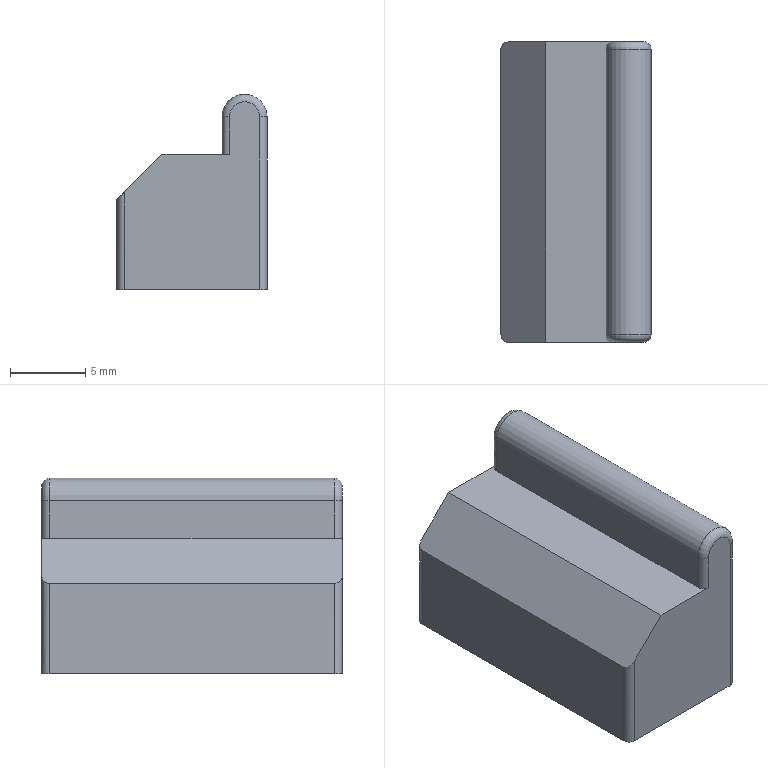NC program | Mastercam | posted with a generic post | part box 10 x 20 x 13 mm
Lines 1 to 867 of 2366:
%
:0001()
(MATERIAL - ALUMINUM MM - 2024)
(T24|100 FEM |H24)
(T9|10 FEM |H9|XY STOCK TO LEAVE - .1|Z STOCK TO LEAVE - 0.)
(T10|10 FEM |H10)
(T5|4 CHM |H5)
(T18|8 BNOS |H18)
(T14|4 BM/BNOS |H14)
N100 G21
N102 G0 G17 G40 G80 G90 G94 G98
N104 G0 G28 G91 Z0.
N106 G0 G28 X0. Y0.
(100 FEM |TOOL - 24|DIA. OFF. - 24|LEN. - 24|TOOL DIA. - 100.)
N108 T24 M6
N110 G0 G54 G90 X-92.5 Y0. C0. B0. S4000 M3
N112 G43 H24 Z57.
N114 Z9.
N116 G1 Z5.62 F600.
N118 X92.5 F4000.
N120 Z4.24 F600.
N122 X-92.5 F4000.
N124 Z2.86 F600.
N126 X92.5 F4000.
N128 Z1.48 F600.
N130 X-92.5 F4000.
N132 Z.1 F600.
N134 X92.5 F4000.
N136 Z0. F600.
N138 X-92.5 F1000.
N140 G0 Z50.
N142 M5
N144 G0 G28 G91 Z0.
N146 G28
N148 M01
N150 G0 G17 G40 G80 G90 G94 G98
N152 G0 G28 G91 Z0.
(10 FEM |TOOL - 9|DIA. OFF. - 9|LEN. - 9|TOOL DIA. - 10.)
N154 T9 M6
N156 G0 G54 G90 X18.41 Y-11.995 C0. B0. S8000 M3
N158 G43 H9 Z50.
N160 Z1.
N162 G1 Z0. F600.
N164 X14.874 Y-8.46 F4000.
N166 G3 X14.167 Y-8.167 I-.707 J-.707
N168 X13.46 Y-8.46 J-1.
N170 G2 X9.5 Y-10.1 Z-.048 I-3.96 J3.96
N172 G1 X-9.5 Z-.257
N174 G2 X-15.1 Y-4.5 Z-.353 J5.6
N176 G1 Y4.5 Z-.452
N178 G2 X-9.5 Y10.1 Z-.548 I5.6
N180 G1 X9.5 Z-.757
N182 G2 X15.1 Y4.5 Z-.853 J-5.6
N184 G1 Y-4.5 Z-.952
N186 G2 X13.46 Y-8.46 Z-1. I-5.6
N188 X9.5 Y-10.1 Z-1.048 I-3.96 J3.96
N190 G1 X-9.5 Z-1.257
N192 G2 X-15.1 Y-4.5 Z-1.353 J5.6
N194 G1 Y4.5 Z-1.452
N196 G2 X-9.5 Y10.1 Z-1.548 I5.6
N198 G1 X9.5 Z-1.757
N200 G2 X15.1 Y4.5 Z-1.853 J-5.6
N202 G1 Y-4.5 Z-1.952
N204 G2 X13.46 Y-8.46 Z-2. I-5.6
N206 X9.5 Y-10.1 Z-2.048 I-3.96 J3.96
N208 G1 X-9.5 Z-2.257
N210 G2 X-15.1 Y-4.5 Z-2.353 J5.6
N212 G1 Y4.5 Z-2.452
N214 G2 X-9.5 Y10.1 Z-2.548 I5.6
N216 G1 X9.5 Z-2.757
N218 G2 X15.1 Y4.5 Z-2.853 J-5.6
N220 G1 Y-4.5 Z-2.952
N222 G2 X13.46 Y-8.46 Z-3. I-5.6
N224 X9.5 Y-10.1 Z-3.048 I-3.96 J3.96
N226 G1 X-9.5 Z-3.257
N228 G2 X-15.1 Y-4.5 Z-3.353 J5.6
N230 G1 Y4.5 Z-3.452
N232 G2 X-9.5 Y10.1 Z-3.548 I5.6
N234 G1 X9.5 Z-3.757
N236 G2 X15.1 Y4.5 Z-3.853 J-5.6
N238 G1 Y-4.5 Z-3.952
N240 G2 X13.46 Y-8.46 Z-4. I-5.6
N242 X9.5 Y-10.1 Z-4.048 I-3.96 J3.96
N244 G1 X-9.5 Z-4.257
N246 G2 X-15.1 Y-4.5 Z-4.353 J5.6
N248 G1 Y4.5 Z-4.452
N250 G2 X-9.5 Y10.1 Z-4.548 I5.6
N252 G1 X9.5 Z-4.757
N254 G2 X15.1 Y4.5 Z-4.853 J-5.6
N256 G1 Y-4.5 Z-4.952
N258 G2 X13.46 Y-8.46 Z-5. I-5.6
N260 X9.5 Y-10.1 Z-5.048 I-3.96 J3.96
N262 G1 X-9.5 Z-5.257
N264 G2 X-15.1 Y-4.5 Z-5.353 J5.6
N266 G1 Y4.5 Z-5.452
N268 G2 X-9.5 Y10.1 Z-5.548 I5.6
N270 G1 X9.5 Z-5.757
N272 G2 X15.1 Y4.5 Z-5.853 J-5.6
N274 G1 Y-4.5 Z-5.952
N276 G2 X13.46 Y-8.46 Z-6. I-5.6
N278 X9.5 Y-10.1 Z-6.048 I-3.96 J3.96
N280 G1 X-9.5 Z-6.257
N282 G2 X-15.1 Y-4.5 Z-6.353 J5.6
N284 G1 Y4.5 Z-6.452
N286 G2 X-9.5 Y10.1 Z-6.548 I5.6
N288 G1 X9.5 Z-6.757
N290 G2 X15.1 Y4.5 Z-6.853 J-5.6
N292 G1 Y-4.5 Z-6.952
N294 G2 X13.46 Y-8.46 Z-7. I-5.6
N296 X9.5 Y-10.1 Z-7.048 I-3.96 J3.96
N298 G1 X-9.5 Z-7.257
N300 G2 X-15.1 Y-4.5 Z-7.353 J5.6
N302 G1 Y4.5 Z-7.452
N304 G2 X-9.5 Y10.1 Z-7.548 I5.6
N306 G1 X9.5 Z-7.757
N308 G2 X15.1 Y4.5 Z-7.853 J-5.6
N310 G1 Y-4.5 Z-7.952
N312 G2 X13.46 Y-8.46 Z-8. I-5.6
N314 X9.5 Y-10.1 Z-8.048 I-3.96 J3.96
N316 G1 X-9.5 Z-8.257
N318 G2 X-15.1 Y-4.5 Z-8.353 J5.6
N320 G1 Y4.5 Z-8.452
N322 G2 X-9.5 Y10.1 Z-8.548 I5.6
N324 G1 X9.5 Z-8.757
N326 G2 X15.1 Y4.5 Z-8.853 J-5.6
N328 G1 Y-4.5 Z-8.952
N330 G2 X13.46 Y-8.46 Z-9. I-5.6
N332 X9.5 Y-10.1 Z-9.048 I-3.96 J3.96
N334 G1 X-9.5 Z-9.257
N336 G2 X-15.1 Y-4.5 Z-9.353 J5.6
N338 G1 Y4.5 Z-9.452
N340 G2 X-9.5 Y10.1 Z-9.548 I5.6
N342 G1 X9.5 Z-9.757
N344 G2 X15.1 Y4.5 Z-9.853 J-5.6
N346 G1 Y-4.5 Z-9.952
N348 G2 X13.46 Y-8.46 Z-10. I-5.6
N350 X9.5 Y-10.1 Z-10.048 I-3.96 J3.96
N352 G1 X-9.5 Z-10.257
N354 G2 X-15.1 Y-4.5 Z-10.353 J5.6
N356 G1 Y4.5 Z-10.452
N358 G2 X-9.5 Y10.1 Z-10.548 I5.6
N360 G1 X9.5 Z-10.757
N362 G2 X15.1 Y4.5 Z-10.853 J-5.6
N364 G1 Y-4.5 Z-10.952
N366 G2 X13.46 Y-8.46 Z-11. I-5.6
N368 X9.5 Y-10.1 Z-11.048 I-3.96 J3.96
N370 G1 X-9.5 Z-11.257
N372 G2 X-15.1 Y-4.5 Z-11.353 J5.6
N374 G1 Y4.5 Z-11.452
N376 G2 X-9.5 Y10.1 Z-11.548 I5.6
N378 G1 X9.5 Z-11.757
N380 G2 X15.1 Y4.5 Z-11.853 J-5.6
N382 G1 Y-4.5 Z-11.952
N384 G2 X13.46 Y-8.46 Z-12. I-5.6
N386 X9.5 Y-10.1 Z-12.048 I-3.96 J3.96
N388 G1 X-9.5 Z-12.257
N390 G2 X-15.1 Y-4.5 Z-12.353 J5.6
N392 G1 Y4.5 Z-12.452
N394 G2 X-9.5 Y10.1 Z-12.548 I5.6
N396 G1 X9.5 Z-12.757
N398 G2 X15.1 Y4.5 Z-12.853 J-5.6
N400 G1 Y-4.5 Z-12.952
N402 G2 X13.46 Y-8.46 Z-13. I-5.6
N404 X9.5 Y-10.1 Z-13.048 I-3.96 J3.96
N406 G1 X-9.5 Z-13.257
N408 G2 X-15.1 Y-4.5 Z-13.353 J5.6
N410 G1 Y4.5 Z-13.452
N412 G2 X-13.46 Y8.46 Z-13.5 I5.6
N414 X-9.5 Y10.1 I3.96 J-3.96
N416 G1 X9.5
N418 G2 X15.1 Y4.5 J-5.6
N420 G1 Y-4.5
N422 G2 X13.46 Y-8.46 I-5.6
N424 X9.5 Y-10.1 I-3.96 J3.96
N426 G1 X-9.5
N428 G2 X-15.1 Y-4.5 J5.6
N430 G1 Y4.5
N432 G2 X-13.091 Y8.797 I5.6
N434 G3 X-12.732 Y9.564 I-.641 J.767
N436 X-12.965 Y10.206 I-1.
N438 G1 X-16.171 Y14.042
N440 G0 Z50.
N442 M5
N444 G0 G28 G91 Z0.
N446 G28
N448 M01
N450 G0 G17 G40 G80 G90 G94 G98
N452 G0 G28 G91 Z0.
(10 FEM |TOOL - 10|DIA. OFF. - 10|LEN. - 10|TOOL DIA. - 10.)
N454 T10 M6
N456 G0 G54 G90 X16.218 Y-9.803 C0. B0. S6000 M3
N458 G43 H10 Z50.
N460 Z1.
N462 G1 Z-13.5 F600.
N464 X14.803 Y-8.389 F1000.
N466 G3 X14.096 Y-8.096 I-.707 J-.707
N468 X13.389 Y-8.389 J-1.
N470 G2 X9.5 Y-10. I-3.889 J3.889
N472 G1 X-9.5
N474 G2 X-15. Y-4.5 J5.5
N476 G1 Y4.5
N478 G2 X-9.5 Y10. I5.5
N480 G1 X9.5
N482 G2 X15. Y4.5 J-5.5
N484 G1 Y-4.5
N486 G2 X13.389 Y-8.389 I-5.5
N488 X13.02 Y-8.726 I-3.889 J3.889
N490 G3 X12.66 Y-9.494 I.64 J-.768
N492 X12.892 Y-10.134 I1.
N494 G1 X14.172 Y-11.671
N496 G0 Z50.
N498 M5
N500 G0 G28 G91 Z0.
N502 G28
N504 M01
N506 G0 G17 G40 G80 G90 G94 G98
N508 G0 G28 G91 Z0.
(4 CHM |TOOL - 5|DIA. OFF. - 5|LEN. - 5|TOOL DIA. - 4.)
N510 T5 M6
N512 G0 G54 G90 X-5. Y-1. C0. B0. S6000 M3
N514 G43 H5 Z50.
N516 G81 G98 Z-.7 R1. F200.
N518 X5.
N520 G80
N522 X9.9 Y-6.85
N524 Z1.
N526 G1 Z-.75 F600.
N528 Y-6.05 F1000.
N530 G3 X9.5 Y-5.65 I-.4
N532 G1 X-9.5
N534 G2 X-10.65 Y-4.5 J1.15
N536 G1 Y4.5
N538 G2 X-9.5 Y5.65 I1.15
N540 G1 X9.5
N542 G2 X10.65 Y4.5 J-1.15
N544 G1 Y-4.5
N546 G2 X9.5 Y-5.65 I-1.15
N548 G1 X9.
N550 G3 X8.6 Y-6.05 J-.4
N552 G1 Y-6.85
N554 G0 Z50.
N556 M5
N558 G0 G28 G91 Z0.
N560 G28
N562 M01
N564 G0 G17 G40 G80 G90 G94 G98
N566 G0 G28 G91 Z0.
(100 FEM |TOOL - 24|DIA. OFF. - 24|LEN. - 24|TOOL DIA. - 100.)
N568 T24 M6
N570 G0 G54 G90 X-92.5 Y0. C0. B0. S4000 M3
N572 G43 H24 Z57.
N574 Z9.
N576 G1 Z5.62 F600.
N578 X92.5 F4000.
N580 Z4.24 F600.
N582 X-92.5 F4000.
N584 Z2.86 F600.
N586 X92.5 F4000.
N588 Z1.48 F600.
N590 X-92.5 F4000.
N592 Z.1 F600.
N594 X92.5 F4000.
N596 Z0. F600.
N598 X-92.5 F1000.
N600 G0 Z50.
N602 M5
N604 G0 G28 G91 Z0.
N606 G28
N608 M01
N610 G0 G17 G40 G80 G90 G94 G98
N612 G0 G28 G91 Z0.
(10 FEM |TOOL - 9|DIA. OFF. - 9|LEN. - 9|TOOL DIA. - 10.)
N614 T9 M6
N616 G0 G54 G90 X18.1 Y3.5 C0. B0. S8000 M3
N618 G43 H9 Z50.
N620 Z1.
N622 G1 Z-.65 F600.
N624 X16.1 F3500.
N626 G3 X15.1 Y2.5 J-1.
N628 G2 X9.5 Y-3.1 I-5.6
N630 G1 X-9.5
N632 G2 X-15.1 Y2.5 J5.6
N634 G3 X-16.1 Y3.5 I-1.
N636 G1 X-18.1
N638 Z-1.3 F600.
N640 X-16.1 F3500.
N642 G2 X-15.1 Y2.5 J-1.
N644 G3 X-9.5 Y-3.1 I5.6
N646 G1 X9.5
N648 G3 X15.1 Y2.5 J5.6
N650 G2 X16.1 Y3.5 I1.
N652 G1 X18.1
N654 Z-1.95 F600.
N656 X16.1 F3500.
N658 G3 X15.1 Y2.5 J-1.
N660 G2 X9.5 Y-3.1 I-5.6
N662 G1 X-9.5
N664 G2 X-15.1 Y2.5 J5.6
N666 G3 X-16.1 Y3.5 I-1.
N668 G1 X-18.1
N670 Z-2.6 F600.
N672 X-16.1 F3500.
N674 G2 X-15.1 Y2.5 J-1.
N676 G3 X-9.5 Y-3.1 I5.6
N678 G1 X9.5
N680 G3 X15.1 Y2.5 J5.6
N682 G2 X16.1 Y3.5 I1.
N684 G1 X18.1
N686 Z-3.25 F600.
N688 X16.1 F3500.
N690 G3 X15.1 Y2.5 J-1.
N692 G2 X9.5 Y-3.1 I-5.6
N694 G1 X-9.5
N696 G2 X-15.1 Y2.5 J5.6
N698 G3 X-16.1 Y3.5 I-1.
N700 G1 X-18.1
N702 Z-3.9 F600.
N704 X-16.1 F3500.
N706 G2 X-15.1 Y2.5 J-1.
N708 G3 X-9.5 Y-3.1 I5.6
N710 G1 X9.5
N712 G3 X15.1 Y2.5 J5.6
N714 G2 X16.1 Y3.5 I1.
N716 G1 X18.1
N718 G0 Z50.
N720 M5
N722 G0 G28 G91 Z0.
N724 G28
N726 M01
N728 G0 G17 G40 G80 G90 G94 G98
N730 G0 G28 G91 Z0.
(10 FEM |TOOL - 10|DIA. OFF. - 10|LEN. - 10|TOOL DIA. - 10.)
N732 T10 M6
N734 G0 G54 G90 X18. Y3.5 C0. B0. S6000 M3
N736 G43 H10 Z50.
N738 Z1.
N740 G1 Z-4. F600.
N742 X16. F1000.
N744 G3 X15. Y2.5 J-1.
N746 G2 X9.5 Y-3. I-5.5
N748 G1 X-9.5
N750 G2 X-15. Y2.5 J5.5
N752 G3 X-16. Y3.5 I-1.
N754 G1 X-18.
N756 G0 Z50.
N758 M5
N760 G0 G28 G91 Z0.
N762 G28
N764 M01
N766 G0 G17 G40 G80 G90 G94 G98
N768 G0 G28 G91 Z0.
(8 BNOS |TOOL - 18|DIA. OFF. - 18|LEN. - 18|TOOL DIA. - 8.)
N770 T18 M6
N772 G0 G54 G90 X-13.5 Y-8.707 C0. B0. S8000 M3
N774 G43 H18 Z50.
N776 Z-2.293
N778 G1 Z-7.293 F600.
N780 X-9.5 F4000.
N782 X9.5
N784 X13.5
N786 Z-7.223
N788 X13.741 Y-8.637
N790 X9.741
N792 X-9.747
N794 X-13.747
N796 Z-7.153
N798 X-13.844 Y-8.568
N800 X-9.844
N802 X9.843
N804 X13.843
N806 Z-7.084
N808 X13.899 Y-8.498
N810 X9.899
N812 X-9.901
N814 X-13.901
N816 Z-7.014
N818 X-13.946 Y-8.428
N820 X-9.946
N822 X9.949
N824 X13.949
N826 Z-6.944
N828 X13.967 Y-8.358
N830 X9.967
N832 X-9.963
N834 X-13.963
N836 Z-6.874
N838 X-13.98 Y-8.289
N840 X-9.98
N842 X9.982
N844 X13.982
N846 Z-6.805
N848 X13.997 Y-8.219
N850 X9.997
N852 X-9.997
N854 X-13.997
N856 Z-6.735
N858 X-14. Y-8.149
N860 X-10.
N862 X10.
N864 X14.
N866 Z-6.665
N868 Y-8.079
N870 X10.
N872 X-10.
N874 X-14.
N876 Z-6.595
N878 Y-8.009
N880 X-10.
N882 X10.
N884 X14.
N886 Z-6.525
N888 Y-7.94
N890 X10.
N892 X-10.
N894 X-14.
N896 Z-6.456
N898 Y-7.87
N900 X-10.
N902 X10.
N904 X14.
N906 Z-6.386
N908 Y-7.8
N910 X10.
N912 X-10.
N914 X-14.
N916 Z-6.316
N918 Y-7.73
N920 X-10.
N922 X10.
N924 X14.
N926 Z-6.246
N928 Y-7.661
N930 X10.
N932 X-10.
N934 X-14.
N936 Z-6.177
N938 Y-7.591
N940 X-10.
N942 X10.
N944 X14.
N946 Z-6.107
N948 Y-7.521
N950 X10.
N952 X-10.
N954 X-14.
N956 Z-6.037
N958 Y-7.451
N960 X-10.
N962 X10.
N964 X14.
N966 Z-5.967
N968 Y-7.382
N970 X10.
N972 X-10.
N974 X-14.
N976 Z-5.898
N978 Y-7.312
N980 X-10.
N982 X10.
N984 X14.
N986 Z-5.828
N988 Y-7.242
N990 X10.
N992 X-10.
N994 X-14.
N996 Z-5.758
N998 Y-7.172
N1000 X-10.
N1002 X10.
N1004 X14.
N1006 Z-5.688
N1008 Y-7.102
N1010 X10.
N1012 X-10.
N1014 X-14.
N1016 Z-5.618
N1018 Y-7.033
N1020 X-10.
N1022 X10.
N1024 X14.
N1026 Z-5.549
N1028 Y-6.963
N1030 X10.
N1032 X-10.
N1034 X-14.
N1036 Z-5.479
N1038 Y-6.893
N1040 X-10.
N1042 X10.
N1044 X14.
N1046 Z-5.409
N1048 Y-6.823
N1050 X10.
N1052 X-10.
N1054 X-14.
N1056 Z-5.339
N1058 Y-6.754
N1060 X-10.
N1062 X10.
N1064 X14.
N1066 Z-5.27
N1068 Y-6.684
N1070 X10.
N1072 X-10.
N1074 X-14.
N1076 Z-5.2
N1078 Y-6.614
N1080 X-10.
N1082 X10.
N1084 X14.
N1086 Z-5.13
N1088 Y-6.544
N1090 X10.
N1092 X-10.
N1094 X-14.
N1096 Z-5.06
N1098 Y-6.475
N1100 X-10.
N1102 X10.
N1104 X14.
N1106 Z-4.991
N1108 Y-6.405
N1110 X10.
N1112 X-10.
N1114 X-14.
N1116 Z-4.921
N1118 Y-6.335
N1120 X-10.
N1122 X10.
N1124 X14.
N1126 Z-4.851
N1128 Y-6.265
N1130 X10.
N1132 X-10.
N1134 X-14.
N1136 Z-4.781
N1138 Y-6.195
N1140 X-10.
N1142 X10.
N1144 X14.
N1146 Z-4.711
N1148 Y-6.126
N1150 X10.
N1152 X-10.
N1154 X-14.
N1156 Z-4.642
N1158 Y-6.056
N1160 X-10.
N1162 X10.
N1164 X14.
N1166 Z-4.572
N1168 Y-5.986
N1170 X10.
N1172 X-10.
N1174 X-14.
N1176 Z-4.502
N1178 Y-5.916
N1180 X-10.
N1182 X10.
N1184 X14.
N1186 Z-4.432
N1188 Y-5.847
N1190 X10.
N1192 X-10.
N1194 X-14.
N1196 Z-4.363
N1198 Y-5.777
N1200 X-10.
N1202 X10.
N1204 X14.
N1206 Z-4.293
N1208 Y-5.707
N1210 X10.
N1212 X-10.
N1214 X-14.
N1216 G0 Z.707
N1218 Z50.
N1220 X13.5 Y-2.
N1222 Z2.5
N1224 G1 Z-2.5 F600.
N1226 X9.5 F4000.
N1228 X-9.5
N1230 X-13.5
N1232 Z-2.392
N1234 Y-1.998
N1236 X-9.5
N1238 X9.5
N1240 X13.5
N1242 Z-2.281
N1244 Y-1.99
N1246 X9.5
N1248 X-9.5
N1250 X-13.5
N1252 Z-2.164
N1254 Y-1.977
N1256 X-9.5
N1258 X9.5
N1260 X13.5
N1262 Z-2.044
N1264 Y-1.958
N1266 X9.5
N1268 X-9.5
N1270 X-13.5
N1272 Z-1.919
N1274 Y-1.932
N1276 X-9.5
N1278 X9.5
N1280 X13.5
N1282 Z-1.792
N1284 Y-1.898
N1286 X9.5
N1288 X-9.5
N1290 X-13.5
N1292 Z-1.66
N1294 Y-1.855
N1296 X-9.5
N1298 X9.5
N1300 X13.5
N1302 Z-1.527
N1304 Y-1.803
N1306 X9.5
N1308 X-9.5
N1310 X-13.5
N1312 Z-1.391
N1314 Y-1.741
N1316 X-9.5
N1318 X9.5
N1320 X13.5
N1322 Z-1.254
N1324 Y-1.668
N1326 X9.5
N1328 X-9.5
N1330 X-13.5
N1332 Z-1.118
N1334 Y-1.583
N1336 X-9.5
N1338 X9.5
N1340 X13.5
N1342 Z-.986
N1344 Y-1.49
N1346 X9.5
N1348 X-9.5
N1350 X-13.5
N1352 Z-.881
N1354 Y-1.405
N1356 X-9.5
N1358 X9.5
N1360 X13.5
N1362 Z-.779
N1364 Y-1.313
N1366 X9.5
N1368 X-9.5
N1370 X-13.5
N1372 Z-.679
N1374 Y-1.213
N1376 X-9.5
N1378 X9.5
N1380 X13.5
N1382 Z-.584
N1384 Y-1.105
N1386 X9.5
N1388 X-9.5
N1390 X-13.5
N1392 Z-.492
N1394 Y-.99
N1396 X-9.5
N1398 X9.5
N1400 X13.5
N1402 Z-.406
N1404 Y-.866
N1406 X9.5
N1408 X-9.5
N1410 X-13.5
N1412 Z-.327
N1414 Y-.735
N1416 X-9.5
N1418 X9.5
N1420 X13.5
N1422 Z-.254
N1424 Y-.598
N1426 X9.5
N1428 X-9.5
N1430 X-13.5
N1432 Z-.189
N1434 Y-.454
N1436 X-9.5
N1438 X9.5
N1440 X13.5
N1442 Z-.133
N1444 Y-.304
N1446 X9.5
N1448 X-9.5
N1450 X-13.5
N1452 Z-.086
N1454 Y-.15
N1456 X-9.5
N1458 X9.5
N1460 X13.5
N1462 Z-.049
N1464 Y.009
N1466 X9.5
N1468 X-9.5
N1470 X-13.5
N1472 Z-.022
N1474 Y.171
N1476 X-9.5
N1478 X9.5
N1480 X13.5
N1482 Z-.005
N1484 Y.335
N1486 X9.5
N1488 X-9.5
N1490 X-13.5
N1492 G0 Z4.995
N1494 Z50.
N1496 Y3.5
N1498 Z5.
N1500 G1 Z0. F600.
N1502 X-9.5 F4000.
N1504 X9.5
N1506 X13.5
N1508 G0 Z5.
N1510 Z50.
N1512 Y6.665
N1514 Z4.995
N1516 G1 Z-.005 F600.
N1518 X9.5 F4000.
N1520 X-9.5
N1522 X-13.5
N1524 Y6.829
N1526 Z-.022
N1528 X-9.5
N1530 X9.5
N1532 X13.5
N1534 Y6.991
N1536 Z-.049
N1538 X9.5
N1540 X-9.5
N1542 X-13.5
N1544 Y7.15
N1546 Z-.086
N1548 X-9.5
N1550 X9.5
N1552 X13.5
N1554 Y7.304
N1556 Z-.133
N1558 X9.5
N1560 X-9.5
N1562 X-13.5
N1564 Y7.454
N1566 Z-.189
N1568 X-9.5
N1570 X9.5
N1572 X13.5
N1574 Y7.598
N1576 Z-.254
N1578 X9.5
N1580 X-9.5
N1582 X-13.5
N1584 Y7.735
N1586 Z-.327
N1588 X-9.5
N1590 X9.5
N1592 X13.5
N1594 Y7.866
N1596 Z-.406
N1598 X9.5
N1600 X-9.5
N1602 X-13.5
N1604 Y7.99
N1606 Z-.492
N1608 X-9.5
N1610 X9.5
N1612 X13.5
N1614 Y8.105
N1616 Z-.584
N1618 X9.5
N1620 X-9.5
N1622 X-13.5
N1624 Y8.213
N1626 Z-.679
N1628 X-9.5
N1630 X9.5
N1632 X13.5
N1634 Y8.313
N1636 Z-.779
N1638 X9.5
N1640 X-9.5
N1642 X-13.5
N1644 Y8.405
N1646 Z-.881
N1648 X-9.5
N1650 X9.5
N1652 X13.5
N1654 Y8.49
N1656 Z-.986
N1658 X9.5
N1660 X-9.5
N1662 X-13.5
N1664 Y8.583
N1666 Z-1.118
N1668 X-9.5
N1670 X9.5
N1672 X13.5
N1674 Y8.668
N1676 Z-1.254
N1678 X9.5
N1680 X-9.5
N1682 X-13.5
N1684 Y8.741
N1686 Z-1.391
N1688 X-9.5
N1690 X9.5
N1692 X13.5
N1694 Y8.803
N1696 Z-1.527
N1698 X9.5
N1700 X-9.5
N1702 X-13.5
N1704 Y8.855
N1706 Z-1.66
N1708 X-9.5
N1710 X9.5
N1712 X13.5
N1714 Y8.898
N1716 Z-1.792
N1718 X9.5
N1720 X-9.5
N1722 X-13.5
N1724 Y8.932
N1726 Z-1.919
N1728 X-9.5
N1730 X9.5
N1732 X13.5
N1734 Y8.958
N1736 Z-2.044
N1738 X9.5
N1740 X-9.5
N1742 X-13.5
N1744 Y8.977
N1746 Z-2.164
N1748 X-9.5
N1750 X9.5
N1752 X13.5
N1754 Y8.99
N1756 Z-2.281
N1758 X9.5
N1760 X-9.5
N1762 X-13.5
N1764 Y8.998
N1766 Z-2.392
N1768 X-9.5
N1770 X9.5
N1772 X13.5
N1774 Y9.
N1776 Z-2.5
N1778 X9.5
N1780 X-9.5
N1782 X-13.5
N1784 G0 Z2.5
N1786 Z50.
N1788 M5
N1790 G0 G28 G91 Z0.
N1792 G28
N1794 M01
N1796 G0 G17 G40 G80 G90 G94 G98
N1798 G0 G28 G91 Z0.